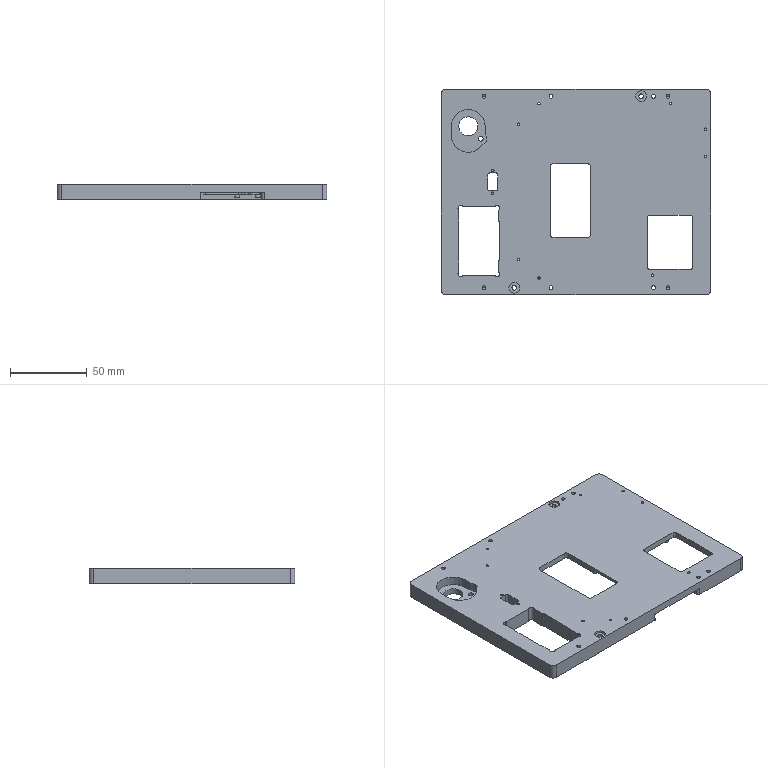NC program | NX | posted with a generic post | part box 176 x 134 x 10 mm
Lines 5447 to 6233 of 8914:
(ZLEVEL_PROFILE_COPY_COPY_COPY_1_COPY_COPY_1_COPY_COPY_COPY_1_COPY_COPY_COPY_CO)
N10814 T19 M6
N10816 G54
N10818 G17 G0 G90 X-53.704 Y2.212 S9500 M3
N10820 G43 Z30. H19
N10822 Z-0.2
N10824 G94 G1 X-53.531 Y1.912 F1000.
N10826 G3 X-53.358 Y1.812 R0.2
N10828 G1 X-52.309 Y1.811 F1100.
N10830 G3 X-52.059 Y2.06 R0.25
N10832 G1 X-52.058 Y3.109
N10834 G3 X-52.158 Y3.283 R0.2
N10836 G1 X-52.458 Y3.456
N10838 G0 X-53.704 Y2.212 Z-0.4
N10840 G1 X-53.531 Y1.912 F1000.
N10842 G3 X-53.358 Y1.812 R0.2
N10844 G1 X-52.309 Y1.811 F1100.
N10846 G3 X-52.059 Y2.06 R0.25
N10848 G1 X-52.058 Y3.109
N10850 G3 X-52.158 Y3.283 R0.2
N10852 G1 X-52.458 Y3.456
N10854 G0 X-53.704 Y2.212 Z-0.6
N10856 G1 X-53.531 Y1.912 F1000.
N10858 G3 X-53.358 Y1.812 R0.2
N10860 G1 X-52.309 Y1.811 F1100.
N10862 G3 X-52.059 Y2.06 R0.25
N10864 G1 X-52.058 Y3.109
N10866 G3 X-52.158 Y3.283 R0.2
N10868 G1 X-52.458 Y3.456
N10870 G0 X-53.704 Y2.212 Z-0.8
N10872 G1 X-53.531 Y1.912 F1000.
N10874 G3 X-53.358 Y1.812 R0.2
N10876 G1 X-52.309 Y1.811 F1100.
N10878 G3 X-52.059 Y2.06 R0.25
N10880 G1 X-52.058 Y3.109
N10882 G3 X-52.158 Y3.283 R0.2
N10884 G1 X-52.458 Y3.456
N10886 G0 X-53.704 Y2.212 Z-1.
N10888 G1 X-53.531 Y1.912 F1000.
N10890 G3 X-53.358 Y1.812 R0.2
N10892 G1 X-52.309 Y1.811 F1100.
N10894 G3 X-52.059 Y2.06 R0.25
N10896 G1 X-52.058 Y3.109
N10898 G3 X-52.158 Y3.283 R0.2
N10900 G1 X-52.458 Y3.456
N10902 G0 X-53.704 Y2.212 Z-1.2
N10904 G1 X-53.531 Y1.912 F1000.
N10906 G3 X-53.358 Y1.812 R0.2
N10908 G1 X-52.309 Y1.811 F1100.
N10910 G3 X-52.059 Y2.06 R0.25
N10912 G1 X-52.058 Y3.109
N10914 G3 X-52.158 Y3.283 R0.2
N10916 G1 X-52.458 Y3.456
N10918 G0 X-53.704 Y2.212 Z-1.4
N10920 G1 X-53.531 Y1.912 F1000.
N10922 G3 X-53.358 Y1.812 R0.2
N10924 G1 X-52.309 Y1.811 F1100.
N10926 G3 X-52.059 Y2.06 R0.25
N10928 G1 X-52.058 Y3.109
N10930 G3 X-52.158 Y3.283 R0.2
N10932 G1 X-52.458 Y3.456
N10934 G0 X-53.704 Y2.212 Z-1.6
N10936 G1 X-53.531 Y1.912 F1000.
N10938 G3 X-53.358 Y1.812 R0.2
N10940 G1 X-52.309 Y1.811 F1100.
N10942 G3 X-52.059 Y2.06 R0.25
N10944 G1 X-52.058 Y3.109
N10946 G3 X-52.158 Y3.283 R0.2
N10948 G1 X-52.458 Y3.456
N10950 G0 X-53.704 Y2.212 Z-1.8
N10952 G1 X-53.531 Y1.912 F1000.
N10954 G3 X-53.358 Y1.812 R0.2
N10956 G1 X-52.309 Y1.811 F1100.
N10958 G3 X-52.059 Y2.06 R0.25
N10960 G1 X-52.058 Y3.109
N10962 G3 X-52.158 Y3.283 R0.2
N10964 G1 X-52.458 Y3.456
N10966 G0 X-53.704 Y2.212 Z-2.
N10968 G1 X-53.531 Y1.912 F1000.
N10970 G3 X-53.358 Y1.812 R0.2
N10972 G1 X-52.309 Y1.811 F1100.
N10974 G3 X-52.059 Y2.06 R0.25
N10976 G1 X-52.058 Y3.109
N10978 G3 X-52.158 Y3.283 R0.2
N10980 G1 X-52.458 Y3.456
N10982 G0 X-53.704 Y2.212 Z-2.2
N10984 G1 X-53.531 Y1.912 F1000.
N10986 G3 X-53.358 Y1.812 R0.2
N10988 G1 X-52.309 Y1.811 F1100.
N10990 G3 X-52.059 Y2.06 R0.25
N10992 G1 X-52.058 Y3.109
N10994 G3 X-52.158 Y3.283 R0.2
N10996 G1 X-52.458 Y3.456
N10998 G0 X-53.704 Y2.212 Z-2.4
N11000 G1 X-53.531 Y1.912 F1000.
N11002 G3 X-53.358 Y1.812 R0.2
N11004 G1 X-52.309 Y1.811 F1100.
N11006 G3 X-52.059 Y2.06 R0.25
N11008 G1 X-52.058 Y3.109
N11010 G3 X-52.158 Y3.283 R0.2
N11012 G1 X-52.458 Y3.456
N11014 G0 X-53.704 Y2.212 Z-2.6
N11016 G1 X-53.531 Y1.912 F1000.
N11018 G3 X-53.358 Y1.812 R0.2
N11020 G1 X-52.309 Y1.811 F1100.
N11022 G3 X-52.059 Y2.06 R0.25
N11024 G1 X-52.058 Y3.109
N11026 G3 X-52.158 Y3.283 R0.2
N11028 G1 X-52.458 Y3.456
N11030 G0 X-53.704 Y2.212 Z-2.8
N11032 G1 X-53.531 Y1.912 F1000.
N11034 G3 X-53.358 Y1.812 R0.2
N11036 G1 X-52.309 Y1.811 F1100.
N11038 G3 X-52.059 Y2.06 R0.25
N11040 G1 X-52.058 Y3.109
N11042 G3 X-52.158 Y3.283 R0.2
N11044 G1 X-52.458 Y3.456
N11046 G0 X-53.704 Y2.212 Z-3.
N11048 G1 X-53.531 Y1.912 F1000.
N11050 G3 X-53.358 Y1.812 R0.2
N11052 G1 X-52.309 Y1.811 F1100.
N11054 G3 X-52.059 Y2.06 R0.25
N11056 G1 X-52.058 Y3.109
N11058 G3 X-52.158 Y3.283 R0.2
N11060 G1 X-52.458 Y3.456
N11062 G0 X-53.704 Y2.212 Z-3.2
N11064 G1 X-53.531 Y1.912 F1000.
N11066 G3 X-53.358 Y1.812 R0.2
N11068 G1 X-52.309 Y1.811 F1100.
N11070 G3 X-52.059 Y2.06 R0.25
N11072 G1 X-52.058 Y3.109
N11074 G3 X-52.158 Y3.283 R0.2
N11076 G1 X-52.458 Y3.456
N11078 G0 X-53.704 Y2.212 Z-3.4
N11080 G1 X-53.531 Y1.912 F1000.
N11082 G3 X-53.358 Y1.812 R0.2
N11084 G1 X-52.309 Y1.811 F1100.
N11086 G3 X-52.059 Y2.06 R0.25
N11088 G1 X-52.058 Y3.109
N11090 G3 X-52.158 Y3.283 R0.2
N11092 G1 X-52.458 Y3.456
N11094 G0 X-53.704 Y2.212 Z-3.6
N11096 G1 X-53.531 Y1.912 F1000.
N11098 G3 X-53.358 Y1.812 R0.2
N11100 G1 X-52.309 Y1.811 F1100.
N11102 G3 X-52.059 Y2.06 R0.25
N11104 G1 X-52.058 Y3.109
N11106 G3 X-52.158 Y3.283 R0.2
N11108 G1 X-52.458 Y3.456
N11110 G0 X-53.704 Y2.212 Z-3.8
N11112 G1 X-53.531 Y1.912 F1000.
N11114 G3 X-53.358 Y1.812 R0.2
N11116 G1 X-52.309 Y1.811 F1100.
N11118 G3 X-52.059 Y2.06 R0.25
N11120 G1 X-52.058 Y3.109
N11122 G3 X-52.158 Y3.283 R0.2
N11124 G1 X-52.458 Y3.456
N11126 G0 X-53.704 Y2.212 Z-4.
N11128 G1 X-53.531 Y1.912 F1000.
N11130 G3 X-53.358 Y1.812 R0.2
N11132 G1 X-52.309 Y1.811 F1100.
N11134 G3 X-52.059 Y2.06 R0.25
N11136 G1 X-52.058 Y3.109
N11138 G3 X-52.158 Y3.283 R0.2
N11140 G1 X-52.458 Y3.456
N11142 G0 X-53.704 Y2.212 Z-4.2
N11144 G1 X-53.531 Y1.912 F1000.
N11146 G3 X-53.358 Y1.812 R0.2
N11148 G1 X-52.309 Y1.811 F1100.
N11150 G3 X-52.059 Y2.06 R0.25
N11152 G1 X-52.058 Y3.109
N11154 G3 X-52.158 Y3.283 R0.2
N11156 G1 X-52.458 Y3.456
N11158 G0 X-53.704 Y2.212 Z-4.4
N11160 G1 X-53.531 Y1.912 F1000.
N11162 G3 X-53.358 Y1.812 R0.2
N11164 G1 X-52.309 Y1.811 F1100.
N11166 G3 X-52.059 Y2.06 R0.25
N11168 G1 X-52.058 Y3.109
N11170 G3 X-52.158 Y3.283 R0.2
N11172 G1 X-52.458 Y3.456
N11174 G0 X-53.704 Y2.212 Z-4.6
N11176 G1 X-53.531 Y1.912 F1000.
N11178 G3 X-53.358 Y1.812 R0.2
N11180 G1 X-52.309 Y1.811 F1100.
N11182 G3 X-52.059 Y2.06 R0.25
N11184 G1 X-52.058 Y3.109
N11186 G3 X-52.158 Y3.283 R0.2
N11188 G1 X-52.458 Y3.456
N11190 G0 X-53.704 Y2.212 Z-4.8
N11192 G1 X-53.531 Y1.912 F1000.
N11194 G3 X-53.358 Y1.812 R0.2
N11196 G1 X-52.309 Y1.811 F1100.
N11198 G3 X-52.059 Y2.06 R0.25
N11200 G1 X-52.058 Y3.109
N11202 G3 X-52.158 Y3.283 R0.2
N11204 G1 X-52.458 Y3.456
N11206 G0 X-53.704 Y2.212 Z-5.
N11208 G1 X-53.531 Y1.912 F1000.
N11210 G3 X-53.358 Y1.812 R0.2
N11212 G1 X-52.309 Y1.811 F1100.
N11214 G3 X-52.059 Y2.06 R0.25
N11216 G1 X-52.058 Y3.109
N11218 G3 X-52.158 Y3.283 R0.2
N11220 G1 X-52.458 Y3.456
N11222 G0 X-53.704 Y2.212 Z-5.2
N11224 G1 X-53.531 Y1.912 F1000.
N11226 G3 X-53.358 Y1.812 R0.2
N11228 G1 X-52.309 Y1.811 F1100.
N11230 G3 X-52.059 Y2.06 R0.25
N11232 G1 X-52.058 Y3.109
N11234 G3 X-52.158 Y3.283 R0.2
N11236 G1 X-52.458 Y3.456
N11238 G0 X-53.704 Y2.212 Z-5.4
N11240 G1 X-53.531 Y1.912 F1000.
N11242 G3 X-53.358 Y1.812 R0.2
N11244 G1 X-52.309 Y1.811 F1100.
N11246 G3 X-52.059 Y2.06 R0.25
N11248 G1 X-52.058 Y3.109
N11250 G3 X-52.158 Y3.283 R0.2
N11252 G1 X-52.458 Y3.456
N11254 G0 X-53.704 Y2.212 Z-5.6
N11256 G1 X-53.531 Y1.912 F1000.
N11258 G3 X-53.358 Y1.812 R0.2
N11260 G1 X-52.309 Y1.811 F1100.
N11262 G3 X-52.059 Y2.06 R0.25
N11264 G1 X-52.058 Y3.109
N11266 G3 X-52.158 Y3.283 R0.2
N11268 G1 X-52.458 Y3.456
N11270 G0 X-53.704 Y2.212 Z-5.8
N11272 G1 X-53.531 Y1.912 F1000.
N11274 G3 X-53.358 Y1.812 R0.2
N11276 G1 X-52.309 Y1.811 F1100.
N11278 G3 X-52.059 Y2.06 R0.25
N11280 G1 X-52.058 Y3.109
N11282 G3 X-52.158 Y3.283 R0.2
N11284 G1 X-52.458 Y3.456
N11286 G0 X-53.704 Y2.212 Z-6.
N11288 G1 X-53.531 Y1.912 F1000.
N11290 G3 X-53.358 Y1.812 R0.2
N11292 G1 X-52.309 Y1.811 F1100.
N11294 G3 X-52.059 Y2.06 R0.25
N11296 G1 X-52.058 Y3.109
N11298 G3 X-52.158 Y3.283 R0.2
N11300 G1 X-52.458 Y3.456
N11302 G0 X-53.704 Y2.212 Z-6.2
N11304 G1 X-53.531 Y1.912 F1000.
N11306 G3 X-53.358 Y1.812 R0.2
N11308 G1 X-52.309 Y1.811 F1100.
N11310 G3 X-52.059 Y2.06 R0.25
N11312 G1 X-52.058 Y3.109
N11314 G3 X-52.158 Y3.283 R0.2
N11316 G1 X-52.458 Y3.456
N11318 G0 X-53.704 Y2.212 Z-6.4
N11320 G1 X-53.531 Y1.912 F1000.
N11322 G3 X-53.358 Y1.812 R0.2
N11324 G1 X-52.309 Y1.811 F1100.
N11326 G3 X-52.059 Y2.06 R0.25
N11328 G1 X-52.058 Y3.109
N11330 G3 X-52.158 Y3.283 R0.2
N11332 G1 X-52.458 Y3.456
N11334 G0 X-53.704 Y2.212 Z-6.6
N11336 G1 X-53.531 Y1.912 F1000.
N11338 G3 X-53.358 Y1.812 R0.2
N11340 G1 X-52.309 Y1.811 F1100.
N11342 G3 X-52.059 Y2.06 R0.25
N11344 G1 X-52.058 Y3.109
N11346 G3 X-52.158 Y3.283 R0.2
N11348 G1 X-52.458 Y3.456
N11350 G0 X-53.704 Y2.212 Z-6.8
N11352 G1 X-53.531 Y1.912 F1000.
N11354 G3 X-53.358 Y1.812 R0.2
N11356 G1 X-52.309 Y1.811 F1100.
N11358 G3 X-52.059 Y2.06 R0.25
N11360 G1 X-52.058 Y3.109
N11362 G3 X-52.158 Y3.283 R0.2
N11364 G1 X-52.458 Y3.456
N11366 G0 X-53.704 Y2.212 Z-7.
N11368 G1 X-53.531 Y1.912 F1000.
N11370 G3 X-53.358 Y1.812 R0.2
N11372 G1 X-52.309 Y1.811 F1100.
N11374 G3 X-52.059 Y2.06 R0.25
N11376 G1 X-52.058 Y3.109
N11378 G3 X-52.158 Y3.283 R0.2
N11380 G1 X-52.458 Y3.456
N11382 G0 X-53.704 Y2.212 Z-7.2
N11384 G1 X-53.531 Y1.912 F1000.
N11386 G3 X-53.358 Y1.812 R0.2
N11388 G1 X-52.309 Y1.811 F1100.
N11390 G3 X-52.059 Y2.06 R0.25
N11392 G1 X-52.058 Y3.109
N11394 G3 X-52.158 Y3.283 R0.2
N11396 G1 X-52.458 Y3.456
N11398 G0 X-53.704 Y2.212 Z-7.4
N11400 G1 X-53.531 Y1.912 F1000.
N11402 G3 X-53.358 Y1.812 R0.2
N11404 G1 X-52.309 Y1.811 F1100.
N11406 G3 X-52.059 Y2.06 R0.25
N11408 G1 X-52.058 Y3.109
N11410 G3 X-52.158 Y3.283 R0.2
N11412 G1 X-52.458 Y3.456
N11414 G0 X-53.704 Y2.212 Z-7.6
N11416 G1 X-53.531 Y1.912 F1000.
N11418 G3 X-53.358 Y1.812 R0.2
N11420 G1 X-52.309 Y1.811 F1100.
N11422 G3 X-52.059 Y2.06 R0.25
N11424 G1 X-52.058 Y3.109
N11426 G3 X-52.158 Y3.283 R0.2
N11428 G1 X-52.458 Y3.456
N11430 G0 X-53.704 Y2.212 Z-7.8
N11432 G1 X-53.531 Y1.912 F1000.
N11434 G3 X-53.358 Y1.812 R0.2
N11436 G1 X-52.309 Y1.811 F1100.
N11438 G3 X-52.059 Y2.06 R0.25
N11440 G1 X-52.058 Y3.109
N11442 G3 X-52.158 Y3.283 R0.2
N11444 G1 X-52.458 Y3.456
N11446 G0 X-53.704 Y2.212 Z-8.
N11448 G1 X-53.531 Y1.912 F1000.
N11450 G3 X-53.358 Y1.812 R0.2
N11452 G1 X-52.309 Y1.811 F1100.
N11454 G3 X-52.059 Y2.06 R0.25
N11456 G1 X-52.058 Y3.109
N11458 G3 X-52.158 Y3.283 R0.2
N11460 G1 X-52.458 Y3.456
N11462 G0 X-53.704 Y2.212 Z-8.2
N11464 G1 X-53.531 Y1.912 F1000.
N11466 G3 X-53.358 Y1.812 R0.2
N11468 G1 X-52.309 Y1.811 F1100.
N11470 G3 X-52.059 Y2.06 R0.25
N11472 G1 X-52.058 Y3.109
N11474 G3 X-52.158 Y3.283 R0.2
N11476 G1 X-52.458 Y3.456
N11478 G0 X-53.704 Y2.212 Z-8.4
N11480 G1 X-53.531 Y1.912 F1000.
N11482 G3 X-53.358 Y1.812 R0.2
N11484 G1 X-52.309 Y1.811 F1100.
N11486 G3 X-52.059 Y2.06 R0.25
N11488 G1 X-52.058 Y3.109
N11490 G3 X-52.158 Y3.283 R0.2
N11492 G1 X-52.458 Y3.456
N11494 G0 X-53.704 Y2.212 Z-8.6
N11496 G1 X-53.531 Y1.912 F1000.
N11498 G3 X-53.358 Y1.812 R0.2
N11500 G1 X-52.309 Y1.811 F1100.
N11502 G3 X-52.059 Y2.06 R0.25
N11504 G1 X-52.058 Y3.109
N11506 G3 X-52.158 Y3.283 R0.2
N11508 G1 X-52.458 Y3.456
N11510 G0 X-53.704 Y2.212 Z-8.8
N11512 G1 X-53.531 Y1.912 F1000.
N11514 G3 X-53.358 Y1.812 R0.2
N11516 G1 X-52.309 Y1.811 F1100.
N11518 G3 X-52.059 Y2.06 R0.25
N11520 G1 X-52.058 Y3.109
N11522 G3 X-52.158 Y3.283 R0.2
N11524 G1 X-52.458 Y3.456
N11526 G0 X-53.704 Y2.212 Z-9.
N11528 G1 X-53.531 Y1.912 F1000.
N11530 G3 X-53.358 Y1.812 R0.2
N11532 G1 X-52.309 Y1.811 F1100.
N11534 G3 X-52.059 Y2.06 R0.25
N11536 G1 X-52.058 Y3.109
N11538 G3 X-52.158 Y3.283 R0.2
N11540 G1 X-52.458 Y3.456
N11542 G0 X-53.704 Y2.212 Z-9.2
N11544 G1 X-53.531 Y1.912 F1000.
N11546 G3 X-53.358 Y1.812 R0.2
N11548 G1 X-52.309 Y1.811 F1100.
N11550 G3 X-52.059 Y2.06 R0.25
N11552 G1 X-52.058 Y3.109
N11554 G3 X-52.158 Y3.283 R0.2
N11556 G1 X-52.458 Y3.456
N11558 G0 X-53.704 Y2.212 Z-9.4
N11560 G1 X-53.531 Y1.912 F1000.
N11562 G3 X-53.358 Y1.812 R0.2
N11564 G1 X-52.309 Y1.811 F1100.
N11566 G3 X-52.059 Y2.06 R0.25
N11568 G1 X-52.058 Y3.109
N11570 G3 X-52.158 Y3.283 R0.2
N11572 G1 X-52.458 Y3.456
N11574 G0 X-53.704 Y2.212 Z-9.6
N11576 G1 X-53.531 Y1.912 F1000.
N11578 G3 X-53.358 Y1.812 R0.2
N11580 G1 X-52.309 Y1.811 F1100.
N11582 G3 X-52.059 Y2.06 R0.25
N11584 G1 X-52.058 Y3.109
N11586 G3 X-52.158 Y3.283 R0.2
N11588 G1 X-52.458 Y3.456
N11590 G0 X-53.704 Y2.212 Z-9.8
N11592 G1 X-53.531 Y1.912 F1000.
N11594 G3 X-53.358 Y1.812 R0.2
N11596 G1 X-52.309 Y1.811 F1100.
N11598 G3 X-52.059 Y2.06 R0.25
N11600 G1 X-52.058 Y3.109
N11602 G3 X-52.158 Y3.283 R0.2
N11604 G1 X-52.458 Y3.456
N11606 G0 X-53.704 Y2.212 Z-10.
N11608 G1 X-53.531 Y1.912 F1000.
N11610 G3 X-53.358 Y1.812 R0.2
N11612 G1 X-52.309 Y1.811 F1100.
N11614 G3 X-52.059 Y2.06 R0.25
N11616 G1 X-52.058 Y3.109
N11618 G3 X-52.158 Y3.283 R0.2
N11620 G1 X-52.458 Y3.456
N11622 G0 Z30.
N11624 X-52.451 Y9.788
N11626 Z-0.2
N11628 G1 X-52.151 Y9.961 F1000.
N11630 G3 X-52.051 Y10.134 R0.2
N11632 G1 X-52.05 Y11.18 F1100.
N11634 G3 X-52.299 Y11.431 R0.25
N11636 G1 X-53.335 Y11.432
N11638 G3 X-53.509 Y11.332 R0.2
N11640 G1 X-53.682 Y11.032
N11642 G0 X-52.451 Y9.788 Z-0.4
N11644 G1 X-52.151 Y9.961 F1000.
N11646 G3 X-52.051 Y10.134 R0.2
N11648 G1 X-52.05 Y11.18 F1100.
N11650 G3 X-52.299 Y11.431 R0.25
N11652 G1 X-53.336 Y11.432
N11654 G3 X-53.509 Y11.332 R0.2
N11656 G1 X-53.682 Y11.032
N11658 G0 X-52.451 Y9.788 Z-0.6
N11660 G1 X-52.151 Y9.961 F1000.
N11662 G3 X-52.051 Y10.134 R0.2
N11664 G1 X-52.05 Y11.18 F1100.
N11666 G3 X-52.299 Y11.431 R0.25
N11668 G1 X-53.336 Y11.432
N11670 G3 X-53.509 Y11.332 R0.2
N11672 G1 X-53.683 Y11.032
N11674 G0 X-52.451 Y9.788 Z-0.8
N11676 G1 X-52.151 Y9.961 F1000.
N11678 G3 X-52.051 Y10.134 R0.2
N11680 G1 X-52.05 Y11.18 F1100.
N11682 G3 X-52.299 Y11.431 R0.25
N11684 G1 X-53.336 Y11.432
N11686 G3 X-53.509 Y11.332 R0.2
N11688 G1 X-53.683 Y11.032
N11690 G0 X-52.451 Y9.788 Z-1.
N11692 G1 X-52.151 Y9.961 F1000.
N11694 G3 X-52.051 Y10.134 R0.2
N11696 G1 X-52.05 Y11.18 F1100.
N11698 G3 X-52.299 Y11.431 R0.25
N11700 G1 X-53.336 Y11.432
N11702 G3 X-53.509 Y11.332 R0.2
N11704 G1 X-53.683 Y11.032
N11706 G0 X-52.451 Y9.788 Z-1.2
N11708 G1 X-52.151 Y9.961 F1000.
N11710 G3 X-52.051 Y10.134 R0.2
N11712 G1 X-52.05 Y11.18 F1100.
N11714 G3 X-52.299 Y11.431 R0.25
N11716 G1 X-53.336 Y11.432
N11718 G3 X-53.509 Y11.332 R0.2
N11720 G1 X-53.683 Y11.032
N11722 G0 X-52.451 Y9.788 Z-1.4
N11724 G1 X-52.151 Y9.961 F1000.
N11726 G3 X-52.051 Y10.134 R0.2
N11728 G1 X-52.05 Y11.18 F1100.
N11730 G3 X-52.299 Y11.431 R0.25
N11732 G1 X-53.336 Y11.432
N11734 G3 X-53.509 Y11.332 R0.2
N11736 G1 X-53.683 Y11.032
N11738 G0 X-52.451 Y9.788 Z-1.6
N11740 G1 X-52.151 Y9.961 F1000.
N11742 G3 X-52.051 Y10.134 R0.2
N11744 G1 X-52.05 Y11.18 F1100.
N11746 G3 X-52.299 Y11.431 R0.25
N11748 G1 X-53.336 Y11.432
N11750 G3 X-53.51 Y11.332 R0.2
N11752 G1 X-53.683 Y11.032
N11754 G0 X-52.451 Y9.788 Z-1.8
N11756 G1 X-52.151 Y9.961 F1000.
N11758 G3 X-52.051 Y10.134 R0.2
N11760 G1 X-52.05 Y11.18 F1100.
N11762 G3 X-52.299 Y11.431 R0.25
N11764 G1 X-53.336 Y11.432
N11766 G3 X-53.51 Y11.332 R0.2
N11768 G1 X-53.683 Y11.032
N11770 G0 X-52.451 Y9.788 Z-2.
N11772 G1 X-52.151 Y9.961 F1000.
N11774 G3 X-52.051 Y10.134 R0.2
N11776 G1 X-52.05 Y11.18 F1100.
N11778 G3 X-52.299 Y11.431 R0.25
N11780 G1 X-53.336 Y11.432
N11782 G3 X-53.51 Y11.332 R0.2
N11784 G1 X-53.683 Y11.032
N11786 G0 X-52.451 Y9.788 Z-2.2
N11788 G1 X-52.151 Y9.961 F1000.
N11790 G3 X-52.051 Y10.134 R0.2
N11792 G1 X-52.05 Y11.18 F1100.
N11794 G3 X-52.299 Y11.431 R0.25
N11796 G1 X-53.337 Y11.432
N11798 G3 X-53.51 Y11.332 R0.2
N11800 G1 X-53.683 Y11.032
N11802 G0 X-52.451 Y9.788 Z-2.4
N11804 G1 X-52.151 Y9.961 F1000.
N11806 G3 X-52.051 Y10.134 R0.2
N11808 G1 X-52.05 Y11.18 F1100.
N11810 G3 X-52.299 Y11.431 R0.25
N11812 G1 X-53.337 Y11.432
N11814 G3 X-53.51 Y11.332 R0.2
N11816 G1 X-53.683 Y11.032
N11818 G0 X-52.451 Y9.788 Z-2.6
N11820 G1 X-52.151 Y9.961 F1000.
N11822 G3 X-52.051 Y10.134 R0.2
N11824 G1 X-52.05 Y11.18 F1100.
N11826 G3 X-52.299 Y11.431 R0.25
N11828 G1 X-53.337 Y11.432
N11830 G3 X-53.51 Y11.332 R0.2
N11832 G1 X-53.684 Y11.032
N11834 G0 X-52.451 Y9.788 Z-2.8
N11836 G1 X-52.151 Y9.961 F1000.
N11838 G3 X-52.051 Y10.134 R0.2
N11840 G1 X-52.05 Y11.18 F1100.
N11842 G3 X-52.299 Y11.431 R0.25
N11844 G1 X-53.337 Y11.432
N11846 G3 X-53.51 Y11.332 R0.2
N11848 G1 X-53.684 Y11.032
N11850 G0 X-52.451 Y9.788 Z-3.
N11852 G1 X-52.151 Y9.961 F1000.
N11854 G3 X-52.051 Y10.134 R0.2
N11856 G1 X-52.05 Y11.18 F1100.
N11858 G3 X-52.299 Y11.431 R0.25
N11860 G1 X-53.337 Y11.432
N11862 G3 X-53.51 Y11.332 R0.2
N11864 G1 X-53.684 Y11.032
N11866 G0 X-52.451 Y9.788 Z-3.2
N11868 G1 X-52.151 Y9.961 F1000.
N11870 G3 X-52.051 Y10.134 R0.2
N11872 G1 X-52.05 Y11.18 F1100.
N11874 G3 X-52.299 Y11.431 R0.25
N11876 G1 X-53.337 Y11.432
N11878 G3 X-53.51 Y11.332 R0.2
N11880 G1 X-53.684 Y11.032
N11882 G0 X-52.451 Y9.788 Z-3.4
N11884 G1 X-52.151 Y9.961 F1000.
N11886 G3 X-52.051 Y10.134 R0.2
N11888 G1 X-52.05 Y11.18 F1100.
N11890 G3 X-52.299 Y11.431 R0.25
N11892 G1 X-53.337 Y11.432
N11894 G3 X-53.51 Y11.332 R0.2
N11896 G1 X-53.684 Y11.032
N11898 G0 X-52.451 Y9.788 Z-3.6
N11900 G1 X-52.151 Y9.961 F1000.
N11902 G3 X-52.051 Y10.134 R0.2
N11904 G1 X-52.05 Y11.18 F1100.
N11906 G3 X-52.299 Y11.431 R0.25
N11908 G1 X-53.337 Y11.432
N11910 G3 X-53.511 Y11.332 R0.2
N11912 G1 X-53.684 Y11.032
N11914 G0 X-52.451 Y9.788 Z-3.8
N11916 G1 X-52.151 Y9.96 F1000.
N11918 G3 X-52.051 Y10.134 R0.2
N11920 G1 X-52.05 Y11.18 F1100.
N11922 G3 X-52.299 Y11.431 R0.25
N11924 G1 X-53.337 Y11.432
N11926 G3 X-53.511 Y11.332 R0.2
N11928 G1 X-53.684 Y11.032
N11930 G0 X-52.451 Y9.788 Z-4.
N11932 G1 X-52.151 Y9.96 F1000.
N11934 G3 X-52.051 Y10.134 R0.2
N11936 G1 X-52.05 Y11.18 F1100.
N11938 G3 X-52.299 Y11.431 R0.25
N11940 G1 X-53.337 Y11.432
N11942 G3 X-53.511 Y11.332 R0.2
N11944 G1 X-53.684 Y11.032
N11946 G0 X-52.451 Y9.788 Z-4.2
N11948 G1 X-52.151 Y9.96 F1000.
N11950 G3 X-52.051 Y10.134 R0.2
N11952 G1 X-52.05 Y11.18 F1100.
N11954 G3 X-52.299 Y11.431 R0.25
N11956 G1 X-53.338 Y11.432
N11958 G3 X-53.511 Y11.332 R0.2
N11960 G1 X-53.684 Y11.032
N11962 G0 X-52.451 Y9.788 Z-4.4
N11964 G1 X-52.151 Y9.96 F1000.
N11966 G3 X-52.051 Y10.134 R0.2
N11968 G1 X-52.05 Y11.18 F1100.
N11970 G3 X-52.299 Y11.431 R0.25
N11972 G1 X-53.338 Y11.432
N11974 G3 X-53.511 Y11.332 R0.2
N11976 G1 X-53.684 Y11.032
N11978 G0 X-52.451 Y9.787 Z-4.6
N11980 G1 X-52.151 Y9.96 F1000.
N11982 G3 X-52.051 Y10.133 R0.2
N11984 G1 X-52.05 Y11.18 F1100.
N11986 G3 X-52.299 Y11.431 R0.25
N11988 G1 X-53.338 Y11.432
N11990 G3 X-53.511 Y11.332 R0.2
N11992 G1 X-53.685 Y11.032
N11994 G0 X-52.451 Y9.787 Z-4.8
N11996 G1 X-52.151 Y9.96 F1000.
N11998 G3 X-52.051 Y10.133 R0.2
N12000 G1 X-52.05 Y11.18 F1100.
N12002 G3 X-52.299 Y11.431 R0.25
N12004 G1 X-53.338 Y11.432
N12006 G3 X-53.511 Y11.332 R0.2
N12008 G1 X-53.685 Y11.032
N12010 G0 X-52.451 Y9.787 Z-5.
N12012 G1 X-52.151 Y9.96 F1000.
N12014 G3 X-52.051 Y10.133 R0.2
N12016 G1 X-52.05 Y11.18 F1100.
N12018 G3 X-52.299 Y11.431 R0.25
N12020 G1 X-53.338 Y11.432
N12022 G3 X-53.511 Y11.332 R0.2
N12024 G1 X-53.685 Y11.032
N12026 G0 X-52.451 Y9.787 Z-5.2
N12028 G1 X-52.151 Y9.96 F1000.
N12030 G3 X-52.051 Y10.133 R0.2
N12032 G1 X-52.05 Y11.18 F1100.
N12034 G3 X-52.299 Y11.431 R0.25
N12036 G1 X-53.338 Y11.432
N12038 G3 X-53.511 Y11.332 R0.2
N12040 G1 X-53.685 Y11.032
N12042 G0 X-52.451 Y9.787 Z-5.4
N12044 G1 X-52.151 Y9.96 F1000.
N12046 G3 X-52.051 Y10.133 R0.2
N12048 G1 X-52.05 Y11.18 F1100.
N12050 G3 X-52.299 Y11.431 R0.25
N12052 G1 X-53.338 Y11.432
N12054 G3 X-53.511 Y11.332 R0.2
N12056 G1 X-53.685 Y11.032
N12058 G0 X-52.451 Y9.787 Z-5.6
N12060 G1 X-52.151 Y9.96 F1000.
N12062 G3 X-52.051 Y10.133 R0.2
N12064 G1 X-52.05 Y11.18 F1100.
N12066 G3 X-52.299 Y11.431 R0.25
N12068 G1 X-53.338 Y11.432
N12070 G3 X-53.512 Y11.332 R0.2
N12072 G1 X-53.685 Y11.032
N12074 G0 X-52.451 Y9.787 Z-5.8
N12076 G1 X-52.151 Y9.96 F1000.
N12078 G3 X-52.051 Y10.133 R0.2
N12080 G1 X-52.05 Y11.18 F1100.
N12082 G3 X-52.299 Y11.431 R0.25
N12084 G1 X-53.338 Y11.432
N12086 G3 X-53.512 Y11.332 R0.2
N12088 G1 X-53.685 Y11.032
N12090 G0 X-52.451 Y9.787 Z-6.
N12092 G1 X-52.151 Y9.96 F1000.
N12094 G3 X-52.051 Y10.133 R0.2
N12096 G1 X-52.05 Y11.18 F1100.
N12098 G3 X-52.299 Y11.431 R0.25
N12100 G1 X-53.338 Y11.432
N12102 G3 X-53.512 Y11.332 R0.2
N12104 G1 X-53.685 Y11.032
N12106 G0 X-52.451 Y9.787 Z-6.2
N12108 G1 X-52.151 Y9.96 F1000.
N12110 G3 X-52.051 Y10.133 R0.2
N12112 G1 X-52.05 Y11.18 F1100.
N12114 G3 X-52.299 Y11.431 R0.25
N12116 G1 X-53.339 Y11.432
N12118 G3 X-53.512 Y11.332 R0.2
N12120 G1 X-53.685 Y11.032
N12122 G0 X-52.451 Y9.787 Z-6.4
N12124 G1 X-52.151 Y9.96 F1000.
N12126 G3 X-52.051 Y10.133 R0.2
N12128 G1 X-52.05 Y11.18 F1100.
N12130 G3 X-52.299 Y11.431 R0.25
N12132 G1 X-53.339 Y11.432
N12134 G3 X-53.512 Y11.332 R0.2
N12136 G1 X-53.686 Y11.032
N12138 G0 X-52.451 Y9.787 Z-6.6
N12140 G1 X-52.151 Y9.96 F1000.
N12142 G3 X-52.051 Y10.133 R0.2
N12144 G1 X-52.05 Y11.18 F1100.
N12146 G3 X-52.299 Y11.431 R0.25
N12148 G1 X-53.339 Y11.432
N12150 G3 X-53.512 Y11.332 R0.2
N12152 G1 X-53.686 Y11.032
N12154 G0 X-52.451 Y9.787 Z-6.8
N12156 G1 X-52.151 Y9.96 F1000.
N12158 G3 X-52.051 Y10.133 R0.2
N12160 G1 X-52.05 Y11.18 F1100.
N12162 G3 X-52.299 Y11.431 R0.25
N12164 G1 X-53.339 Y11.432
N12166 G3 X-53.512 Y11.332 R0.2
N12168 G1 X-53.686 Y11.032
N12170 G0 X-52.451 Y9.787 Z-7.
N12172 G1 X-52.151 Y9.96 F1000.
N12174 G3 X-52.051 Y10.133 R0.2
N12176 G1 X-52.05 Y11.18 F1100.
N12178 G3 X-52.299 Y11.431 R0.25
N12180 G1 X-53.339 Y11.432
N12182 G3 X-53.512 Y11.332 R0.2
N12184 G1 X-53.686 Y11.032
N12186 G0 X-52.451 Y9.787 Z-7.2
N12188 G1 X-52.151 Y9.96 F1000.
N12190 G3 X-52.051 Y10.133 R0.2
N12192 G1 X-52.05 Y11.18 F1100.
N12194 G3 X-52.299 Y11.431 R0.25
N12196 G1 X-53.339 Y11.432
N12198 G3 X-53.512 Y11.332 R0.2
N12200 G1 X-53.686 Y11.032
N12202 G0 X-52.451 Y9.787 Z-7.4
N12204 G1 X-52.151 Y9.96 F1000.
N12206 G3 X-52.051 Y10.133 R0.2
N12208 G1 X-52.05 Y11.18 F1100.
N12210 G3 X-52.299 Y11.431 R0.25
N12212 G1 X-53.339 Y11.432
N12214 G3 X-53.513 Y11.332 R0.2
N12216 G1 X-53.686 Y11.032
N12218 G0 X-52.451 Y9.787 Z-7.6
N12220 G1 X-52.151 Y9.96 F1000.
N12222 G3 X-52.051 Y10.133 R0.2
N12224 G1 X-52.05 Y11.18 F1100.
N12226 G3 X-52.299 Y11.431 R0.25
N12228 G1 X-53.339 Y11.432
N12230 G3 X-53.513 Y11.332 R0.2
N12232 G1 X-53.686 Y11.032
N12234 G0 X-52.451 Y9.787 Z-7.8
N12236 G1 X-52.151 Y9.96 F1000.
N12238 G3 X-52.051 Y10.133 R0.2
N12240 G1 X-52.05 Y11.18 F1100.
N12242 G3 X-52.299 Y11.431 R0.25
N12244 G1 X-53.339 Y11.432
N12246 G3 X-53.513 Y11.332 R0.2
N12248 G1 X-53.686 Y11.032
N12250 G0 X-52.451 Y9.787 Z-8.
N12252 G1 X-52.151 Y9.96 F1000.
N12254 G3 X-52.051 Y10.133 R0.2
N12256 G1 X-52.05 Y11.18 F1100.
N12258 G3 X-52.299 Y11.431 R0.25
N12260 G1 X-53.34 Y11.432
N12262 G3 X-53.513 Y11.332 R0.2
N12264 G1 X-53.686 Y11.032
N12266 G0 X-52.451 Y9.787 Z-8.2
N12268 G1 X-52.151 Y9.96 F1000.
N12270 G3 X-52.051 Y10.133 R0.2
N12272 G1 X-52.05 Y11.18 F1100.
N12274 G3 X-52.299 Y11.431 R0.25
N12276 G1 X-53.34 Y11.432
N12278 G3 X-53.513 Y11.332 R0.2
N12280 G1 X-53.686 Y11.032
N12282 G0 X-52.451 Y9.787 Z-8.4
N12284 G1 X-52.151 Y9.96 F1000.
N12286 G3 X-52.051 Y10.133 R0.2
N12288 G1 X-52.05 Y11.18 F1100.
N12290 G3 X-52.299 Y11.431 R0.25
N12292 G1 X-53.34 Y11.432
N12294 G3 X-53.513 Y11.332 R0.2
N12296 G1 X-53.687 Y11.032
N12298 G0 X-52.451 Y9.787 Z-8.6
N12300 G1 X-52.151 Y9.96 F1000.
N12302 G3 X-52.051 Y10.133 R0.2
N12304 G1 X-52.05 Y11.18 F1100.
N12306 G3 X-52.299 Y11.431 R0.25
N12308 G1 X-53.34 Y11.432
N12310 G3 X-53.513 Y11.332 R0.2
N12312 G1 X-53.687 Y11.032
N12314 G0 X-52.451 Y9.787 Z-8.8
N12316 G1 X-52.151 Y9.96 F1000.
N12318 G3 X-52.051 Y10.133 R0.2
N12320 G1 X-52.05 Y11.18 F1100.
N12322 G3 X-52.299 Y11.431 R0.25
N12324 G1 X-53.34 Y11.432
N12326 G3 X-53.513 Y11.332 R0.2
N12328 G1 X-53.687 Y11.032
N12330 G0 X-52.451 Y9.787 Z-9.
N12332 G1 X-52.151 Y9.96 F1000.
N12334 G3 X-52.051 Y10.133 R0.2
N12336 G1 X-52.05 Y11.18 F1100.
N12338 G3 X-52.299 Y11.431 R0.25
N12340 G1 X-53.34 Y11.432
N12342 G3 X-53.513 Y11.332 R0.2
N12344 G1 X-53.687 Y11.032
N12346 G0 X-52.451 Y9.787 Z-9.2
N12348 G1 X-52.151 Y9.96 F1000.
N12350 G3 X-52.051 Y10.133 R0.2
N12352 G1 X-52.05 Y11.18 F1100.
N12354 G3 X-52.299 Y11.431 R0.25
N12356 G1 X-53.34 Y11.432
N12358 G3 X-53.513 Y11.332 R0.2
N12360 G1 X-53.687 Y11.032
N12362 G0 X-52.451 Y9.787 Z-9.4
N12364 G1 X-52.151 Y9.96 F1000.
N12366 G3 X-52.051 Y10.133 R0.2
N12368 G1 X-52.05 Y11.18 F1100.
N12370 G3 X-52.299 Y11.431 R0.25
N12372 G1 X-53.34 Y11.432
N12374 G3 X-53.514 Y11.332 R0.2
N12376 G1 X-53.687 Y11.032
N12378 G0 X-52.451 Y9.787 Z-9.6
N12380 G1 X-52.151 Y9.96 F1000.